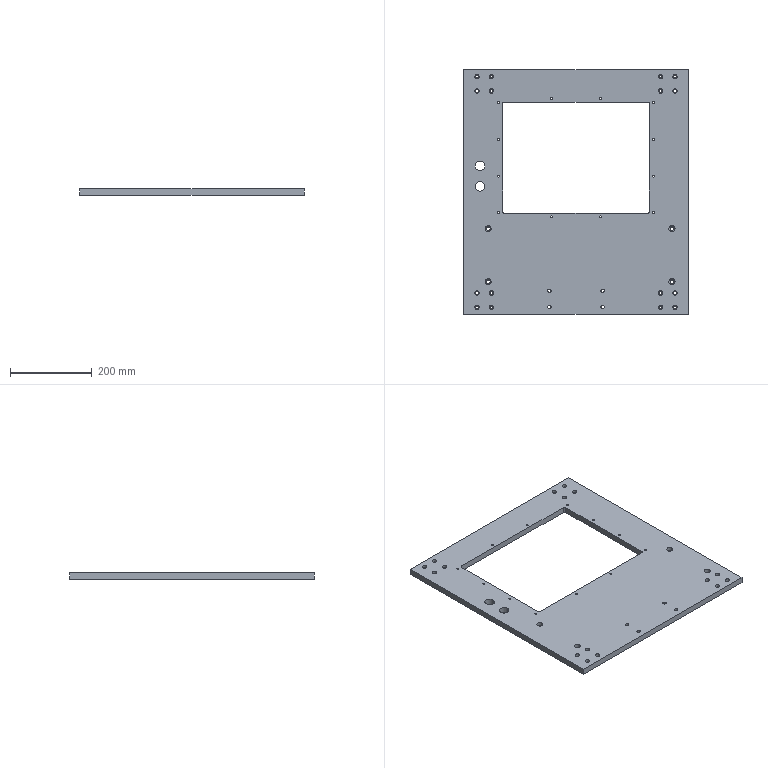Part | SolidWorks | features BaseBody 1, ICE 1 | 1 solid | 150 faces | box 550 x 600 x 15 mm | volume 3438854 mm3 | cylinder 120 | plane 30 | commonest cylinder face diameters 6.6 x32 11 x32 5 x24 8.5 x8 9 x8 15 x8